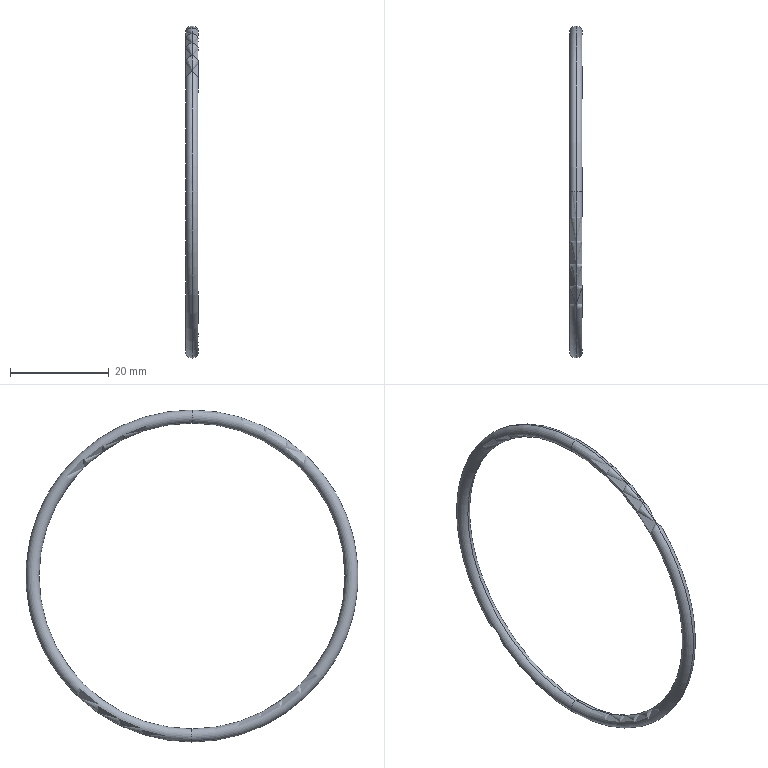Part | SolidWorks | features Revolution 1 | 1 solid | 4 faces | box 2.65 x 67.35 x 67.35 mm | volume 1121 mm3 | torus 4
STEP:
#1=CARTESIAN_POINT('',(5.,0.,-33.675));
#2=VERTEX_POINT('',#1);
#3=CARTESIAN_POINT('',(5.,0.,-31.025));
#4=VERTEX_POINT('',#3);
#5=CARTESIAN_POINT('',(5.,0.,-32.35));
#6=DIRECTION('',(0.,1.,0.));
#7=DIRECTION('',(0.,0.,1.));
#8=AXIS2_PLACEMENT_3D('',#5,#6,#7);
#9=CIRCLE('',#8,1.325);
#10=EDGE_CURVE('',#2,#4,#9,.T.);
#11=ORIENTED_EDGE('',*,*,#10,.F.);
#12=CARTESIAN_POINT('',(5.,0.,33.675));
#13=VERTEX_POINT('',#12);
#14=CARTESIAN_POINT('',(5.,0.,0.));
#15=DIRECTION('',(-1.,0.,0.));
#16=DIRECTION('',(0.,0.,1.));
#17=AXIS2_PLACEMENT_3D('',#14,#15,#16);
#18=CIRCLE('',#17,33.675);
#19=EDGE_CURVE('',#2,#13,#18,.T.);
#20=ORIENTED_EDGE('',*,*,#19,.T.);
#21=CARTESIAN_POINT('',(5.,0.,31.025));
#22=VERTEX_POINT('',#21);
#23=CARTESIAN_POINT('',(5.,0.,32.35));
#24=DIRECTION('',(0.,-1.,0.));
#25=DIRECTION('',(0.,0.,-1.));
#26=AXIS2_PLACEMENT_3D('',#23,#24,#25);
#27=CIRCLE('',#26,1.325);
#28=EDGE_CURVE('',#13,#22,#27,.T.);
#29=ORIENTED_EDGE('',*,*,#28,.T.);
#30=CARTESIAN_POINT('',(5.,0.,0.));
#31=DIRECTION('',(-1.,0.,0.));
#32=DIRECTION('',(0.,0.,1.));
#33=AXIS2_PLACEMENT_3D('',#30,#31,#32);
#34=CIRCLE('',#33,31.025);
#35=EDGE_CURVE('',#4,#22,#34,.T.);
#36=ORIENTED_EDGE('',*,*,#35,.F.);
#37=EDGE_LOOP('',(#11,#20,#29,#36));
#38=FACE_OUTER_BOUND('',#37,.T.);
#39=CARTESIAN_POINT('',(5.,0.,0.));
#40=DIRECTION('',(-1.,0.,0.));
#41=DIRECTION('',(0.,0.,1.));
#42=AXIS2_PLACEMENT_3D('',#39,#40,#41);
#43=TOROIDAL_SURFACE('',#42,32.35,1.325);
#44=ADVANCED_FACE('',(#38),#43,.T.);
#45=ORIENTED_EDGE('',*,*,#28,.F.);
#46=CARTESIAN_POINT('',(5.,0.,0.));
#47=DIRECTION('',(-1.,0.,0.));
#48=DIRECTION('',(0.,0.,1.));
#49=AXIS2_PLACEMENT_3D('',#46,#47,#48);
#50=CIRCLE('',#49,33.675);
#51=EDGE_CURVE('',#13,#2,#50,.T.);
#52=ORIENTED_EDGE('',*,*,#51,.T.);
#53=ORIENTED_EDGE('',*,*,#10,.T.);
#54=CARTESIAN_POINT('',(5.,0.,0.));
#55=DIRECTION('',(-1.,0.,0.));
#56=DIRECTION('',(0.,0.,1.));
#57=AXIS2_PLACEMENT_3D('',#54,#55,#56);
#58=CIRCLE('',#57,31.025);
#59=EDGE_CURVE('',#22,#4,#58,.T.);
#60=ORIENTED_EDGE('',*,*,#59,.F.);
#61=EDGE_LOOP('',(#45,#52,#53,#60));
#62=FACE_OUTER_BOUND('',#61,.T.);
#63=CARTESIAN_POINT('',(5.,0.,0.));
#64=DIRECTION('',(-1.,0.,0.));
#65=DIRECTION('',(0.,0.,1.));
#66=AXIS2_PLACEMENT_3D('',#63,#64,#65);
#67=TOROIDAL_SURFACE('',#66,32.35,1.325);
#68=ADVANCED_FACE('',(#62),#67,.T.);
#69=ORIENTED_EDGE('',*,*,#51,.F.);
#70=CARTESIAN_POINT('',(5.,0.,32.35));
#71=DIRECTION('',(0.,-1.,0.));
#72=DIRECTION('',(0.,0.,-1.));
#73=AXIS2_PLACEMENT_3D('',#70,#71,#72);
#74=CIRCLE('',#73,1.325);
#75=EDGE_CURVE('',#22,#13,#74,.T.);
#76=ORIENTED_EDGE('',*,*,#75,.F.);
#77=ORIENTED_EDGE('',*,*,#59,.T.);
#78=CARTESIAN_POINT('',(5.,0.,-32.35));
#79=DIRECTION('',(0.,1.,0.));
#80=DIRECTION('',(0.,0.,1.));
#81=AXIS2_PLACEMENT_3D('',#78,#79,#80);
#82=CIRCLE('',#81,1.325);
#83=EDGE_CURVE('',#4,#2,#82,.T.);
#84=ORIENTED_EDGE('',*,*,#83,.T.);
#85=EDGE_LOOP('',(#69,#76,#77,#84));
#86=FACE_OUTER_BOUND('',#85,.T.);
#87=CARTESIAN_POINT('',(5.,0.,0.));
#88=DIRECTION('',(-1.,0.,0.));
#89=DIRECTION('',(0.,0.,1.));
#90=AXIS2_PLACEMENT_3D('',#87,#88,#89);
#91=TOROIDAL_SURFACE('',#90,32.35,1.325);
#92=ADVANCED_FACE('',(#86),#91,.T.);
#93=ORIENTED_EDGE('',*,*,#19,.F.);
#94=ORIENTED_EDGE('',*,*,#83,.F.);
#95=ORIENTED_EDGE('',*,*,#35,.T.);
#96=ORIENTED_EDGE('',*,*,#75,.T.);
#97=EDGE_LOOP('',(#93,#94,#95,#96));
#98=FACE_OUTER_BOUND('',#97,.T.);
#99=CARTESIAN_POINT('',(5.,0.,0.));
#100=DIRECTION('',(-1.,0.,0.));
#101=DIRECTION('',(0.,0.,1.));
#102=AXIS2_PLACEMENT_3D('',#99,#100,#101);
#103=TOROIDAL_SURFACE('',#102,32.35,1.325);
#104=ADVANCED_FACE('',(#98),#103,.T.);
#105=CLOSED_SHELL('',(#44,#68,#92,#104));
#106=MANIFOLD_SOLID_BREP('',#105);
#107=CARTESIAN_POINT('',(0.,0.,0.));
#108=DIRECTION('',(0.,0.,1.));
#109=DIRECTION('',(1.,0.,0.));
#110=AXIS2_PLACEMENT_3D('',#107,#108,#109);
#111=(LENGTH_UNIT()NAMED_UNIT(*)SI_UNIT(.MILLI.,.METRE.));
#112=UNCERTAINTY_MEASURE_WITH_UNIT(LENGTH_MEASURE(0.00001),#111,'','');
#113=(NAMED_UNIT(*)PLANE_ANGLE_UNIT()SI_UNIT($,.RADIAN.));
#114=(NAMED_UNIT(*)SI_UNIT($,.STERADIAN.)SOLID_ANGLE_UNIT());
#115=(GEOMETRIC_REPRESENTATION_CONTEXT(3)GLOBAL_UNCERTAINTY_ASSIGNED_CONTEXT((#112))GLOBAL_UNIT_ASSIGNED_CONTEXT((#111,#113,#114))REPRESENTATION_CONTEXT('',''));
#116=ADVANCED_BREP_SHAPE_REPRESENTATION('',(#106,#110),#115);